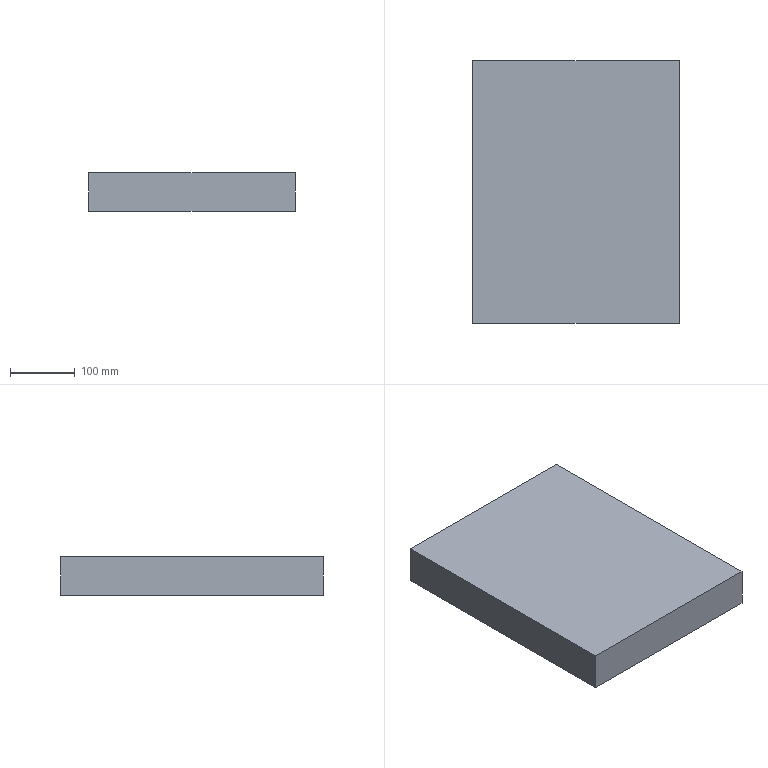Part | STEP file | zhichentai2 | 1 solid | 6 faces | box 320 x 406 x 60 mm | volume 7795200 mm3 | plane 6
STEP:
#1=CARTESIAN_POINT('',(0.,0.,0.));
#2=DIRECTION('',(0.,0.,1.));
#3=DIRECTION('',(1.,0.,0.));
#4=AXIS2_PLACEMENT_3D('',#1,#2,#3);
#5=CARTESIAN_POINT('',(160.,-203.,-30.));
#6=VERTEX_POINT('',#5);
#7=CARTESIAN_POINT('',(160.,203.,-30.));
#8=VERTEX_POINT('',#7);
#9=CARTESIAN_POINT('',(160.,203.,-30.));
#10=DIRECTION('',(0.,1.,0.));
#11=VECTOR('',#10,1.);
#12=LINE('',#9,#11);
#13=CARTESIAN_POINT('',(160.,203.,30.));
#14=DIRECTION('',(-1.,0.,0.));
#15=DIRECTION('',(0.,-1.,0.));
#16=AXIS2_PLACEMENT_3D('',#13,#14,#15);
#17=PLANE('',#16);
#18=CARTESIAN_POINT('',(0.,-60.));
#19=DIRECTION('',(-1.,0.));
#20=VECTOR('',#19,1.);
#21=LINE('',#18,#20);
#22=(GEOMETRIC_REPRESENTATION_CONTEXT(2)PARAMETRIC_REPRESENTATION_CONTEXT()REPRESENTATION_CONTEXT('',''));
#23=DEFINITIONAL_REPRESENTATION('',(#21),#22);
#24=PCURVE('',#17,#23);
#25=CARTESIAN_POINT('',(0.,0.,-30.));
#26=DIRECTION('',(0.,0.,1.));
#27=DIRECTION('',(1.,0.,0.));
#28=AXIS2_PLACEMENT_3D('',#25,#26,#27);
#29=PLANE('',#28);
#30=CARTESIAN_POINT('',(160.,203.));
#31=DIRECTION('',(0.,1.));
#32=VECTOR('',#31,1.);
#33=LINE('',#30,#32);
#34=(GEOMETRIC_REPRESENTATION_CONTEXT(2)PARAMETRIC_REPRESENTATION_CONTEXT()REPRESENTATION_CONTEXT('',''));
#35=DEFINITIONAL_REPRESENTATION('',(#33),#34);
#36=PCURVE('',#29,#35);
#37=SURFACE_CURVE('',#12,(#24,#36),.PCURVE_S1.);
#38=EDGE_CURVE('',#6,#8,#37,.T.);
#39=ORIENTED_EDGE('',*,*,#38,.T.);
#40=CARTESIAN_POINT('',(160.,203.,30.));
#41=VERTEX_POINT('',#40);
#42=CARTESIAN_POINT('',(160.,203.,30.));
#43=DIRECTION('',(0.,0.,-1.));
#44=VECTOR('',#43,1.);
#45=LINE('',#42,#44);
#46=CARTESIAN_POINT('',(0.,0.));
#47=DIRECTION('',(0.,-1.));
#48=VECTOR('',#47,1.);
#49=LINE('',#46,#48);
#50=(GEOMETRIC_REPRESENTATION_CONTEXT(2)PARAMETRIC_REPRESENTATION_CONTEXT()REPRESENTATION_CONTEXT('',''));
#51=DEFINITIONAL_REPRESENTATION('',(#49),#50);
#52=PCURVE('',#17,#51);
#53=CARTESIAN_POINT('',(-160.,203.,30.));
#54=DIRECTION('',(0.,-1.,0.));
#55=DIRECTION('',(0.,0.,-1.));
#56=AXIS2_PLACEMENT_3D('',#53,#54,#55);
#57=PLANE('',#56);
#58=CARTESIAN_POINT('',(0.,320.));
#59=DIRECTION('',(1.,0.));
#60=VECTOR('',#59,1.);
#61=LINE('',#58,#60);
#62=(GEOMETRIC_REPRESENTATION_CONTEXT(2)PARAMETRIC_REPRESENTATION_CONTEXT()REPRESENTATION_CONTEXT('',''));
#63=DEFINITIONAL_REPRESENTATION('',(#61),#62);
#64=PCURVE('',#57,#63);
#65=SURFACE_CURVE('',#45,(#52,#64),.PCURVE_S1.);
#66=EDGE_CURVE('',#41,#8,#65,.T.);
#67=ORIENTED_EDGE('',*,*,#66,.F.);
#68=CARTESIAN_POINT('',(160.,-203.,30.));
#69=VERTEX_POINT('',#68);
#70=CARTESIAN_POINT('',(160.,203.,30.));
#71=DIRECTION('',(0.,1.,0.));
#72=VECTOR('',#71,1.);
#73=LINE('',#70,#72);
#74=CARTESIAN_POINT('',(0.,0.));
#75=DIRECTION('',(-1.,0.));
#76=VECTOR('',#75,1.);
#77=LINE('',#74,#76);
#78=(GEOMETRIC_REPRESENTATION_CONTEXT(2)PARAMETRIC_REPRESENTATION_CONTEXT()REPRESENTATION_CONTEXT('',''));
#79=DEFINITIONAL_REPRESENTATION('',(#77),#78);
#80=PCURVE('',#17,#79);
#81=CARTESIAN_POINT('',(0.,0.,30.));
#82=DIRECTION('',(0.,0.,1.));
#83=DIRECTION('',(1.,0.,0.));
#84=AXIS2_PLACEMENT_3D('',#81,#82,#83);
#85=PLANE('',#84);
#86=CARTESIAN_POINT('',(160.,203.));
#87=DIRECTION('',(0.,1.));
#88=VECTOR('',#87,1.);
#89=LINE('',#86,#88);
#90=(GEOMETRIC_REPRESENTATION_CONTEXT(2)PARAMETRIC_REPRESENTATION_CONTEXT()REPRESENTATION_CONTEXT('',''));
#91=DEFINITIONAL_REPRESENTATION('',(#89),#90);
#92=PCURVE('',#85,#91);
#93=SURFACE_CURVE('',#73,(#80,#92),.PCURVE_S1.);
#94=EDGE_CURVE('',#69,#41,#93,.T.);
#95=ORIENTED_EDGE('',*,*,#94,.F.);
#96=CARTESIAN_POINT('',(160.,-203.,30.));
#97=DIRECTION('',(0.,0.,-1.));
#98=VECTOR('',#97,1.);
#99=LINE('',#96,#98);
#100=CARTESIAN_POINT('',(406.,0.));
#101=DIRECTION('',(0.,-1.));
#102=VECTOR('',#101,1.);
#103=LINE('',#100,#102);
#104=(GEOMETRIC_REPRESENTATION_CONTEXT(2)PARAMETRIC_REPRESENTATION_CONTEXT()REPRESENTATION_CONTEXT('',''));
#105=DEFINITIONAL_REPRESENTATION('',(#103),#104);
#106=PCURVE('',#17,#105);
#107=CARTESIAN_POINT('',(-160.,-203.,30.));
#108=DIRECTION('',(0.,1.,0.));
#109=DIRECTION('',(0.,0.,1.));
#110=AXIS2_PLACEMENT_3D('',#107,#108,#109);
#111=PLANE('',#110);
#112=CARTESIAN_POINT('',(0.,320.));
#113=DIRECTION('',(-1.,0.));
#114=VECTOR('',#113,1.);
#115=LINE('',#112,#114);
#116=(GEOMETRIC_REPRESENTATION_CONTEXT(2)PARAMETRIC_REPRESENTATION_CONTEXT()REPRESENTATION_CONTEXT('',''));
#117=DEFINITIONAL_REPRESENTATION('',(#115),#116);
#118=PCURVE('',#111,#117);
#119=SURFACE_CURVE('',#99,(#106,#118),.PCURVE_S1.);
#120=EDGE_CURVE('',#69,#6,#119,.T.);
#121=ORIENTED_EDGE('',*,*,#120,.T.);
#122=EDGE_LOOP('',(#39,#67,#95,#121));
#123=FACE_BOUND('',#122,.T.);
#124=ADVANCED_FACE('',(#123),#17,.F.);
#125=CARTESIAN_POINT('',(-160.,203.,-30.));
#126=VERTEX_POINT('',#125);
#127=CARTESIAN_POINT('',(-160.,203.,-30.));
#128=DIRECTION('',(-1.,0.,0.));
#129=VECTOR('',#128,1.);
#130=LINE('',#127,#129);
#131=CARTESIAN_POINT('',(60.,0.));
#132=DIRECTION('',(0.,-1.));
#133=VECTOR('',#132,1.);
#134=LINE('',#131,#133);
#135=(GEOMETRIC_REPRESENTATION_CONTEXT(2)PARAMETRIC_REPRESENTATION_CONTEXT()REPRESENTATION_CONTEXT('',''));
#136=DEFINITIONAL_REPRESENTATION('',(#134),#135);
#137=PCURVE('',#57,#136);
#138=CARTESIAN_POINT('',(-160.,203.));
#139=DIRECTION('',(-1.,0.));
#140=VECTOR('',#139,1.);
#141=LINE('',#138,#140);
#142=(GEOMETRIC_REPRESENTATION_CONTEXT(2)PARAMETRIC_REPRESENTATION_CONTEXT()REPRESENTATION_CONTEXT('',''));
#143=DEFINITIONAL_REPRESENTATION('',(#141),#142);
#144=PCURVE('',#29,#143);
#145=SURFACE_CURVE('',#130,(#137,#144),.PCURVE_S1.);
#146=EDGE_CURVE('',#8,#126,#145,.T.);
#147=ORIENTED_EDGE('',*,*,#146,.T.);
#148=CARTESIAN_POINT('',(-160.,203.,30.));
#149=VERTEX_POINT('',#148);
#150=CARTESIAN_POINT('',(-160.,203.,30.));
#151=DIRECTION('',(0.,0.,-1.));
#152=VECTOR('',#151,1.);
#153=LINE('',#150,#152);
#154=CARTESIAN_POINT('',(0.,0.));
#155=DIRECTION('',(1.,0.));
#156=VECTOR('',#155,1.);
#157=LINE('',#154,#156);
#158=(GEOMETRIC_REPRESENTATION_CONTEXT(2)PARAMETRIC_REPRESENTATION_CONTEXT()REPRESENTATION_CONTEXT('',''));
#159=DEFINITIONAL_REPRESENTATION('',(#157),#158);
#160=PCURVE('',#57,#159);
#161=CARTESIAN_POINT('',(-160.,203.,30.));
#162=DIRECTION('',(1.,0.,0.));
#163=DIRECTION('',(0.,1.,0.));
#164=AXIS2_PLACEMENT_3D('',#161,#162,#163);
#165=PLANE('',#164);
#166=CARTESIAN_POINT('',(0.,0.));
#167=DIRECTION('',(0.,-1.));
#168=VECTOR('',#167,1.);
#169=LINE('',#166,#168);
#170=(GEOMETRIC_REPRESENTATION_CONTEXT(2)PARAMETRIC_REPRESENTATION_CONTEXT()REPRESENTATION_CONTEXT('',''));
#171=DEFINITIONAL_REPRESENTATION('',(#169),#170);
#172=PCURVE('',#165,#171);
#173=SURFACE_CURVE('',#153,(#160,#172),.PCURVE_S1.);
#174=EDGE_CURVE('',#149,#126,#173,.T.);
#175=ORIENTED_EDGE('',*,*,#174,.F.);
#176=CARTESIAN_POINT('',(-160.,203.,30.));
#177=DIRECTION('',(-1.,0.,0.));
#178=VECTOR('',#177,1.);
#179=LINE('',#176,#178);
#180=CARTESIAN_POINT('',(0.,0.));
#181=DIRECTION('',(0.,-1.));
#182=VECTOR('',#181,1.);
#183=LINE('',#180,#182);
#184=(GEOMETRIC_REPRESENTATION_CONTEXT(2)PARAMETRIC_REPRESENTATION_CONTEXT()REPRESENTATION_CONTEXT('',''));
#185=DEFINITIONAL_REPRESENTATION('',(#183),#184);
#186=PCURVE('',#57,#185);
#187=CARTESIAN_POINT('',(-160.,203.));
#188=DIRECTION('',(-1.,0.));
#189=VECTOR('',#188,1.);
#190=LINE('',#187,#189);
#191=(GEOMETRIC_REPRESENTATION_CONTEXT(2)PARAMETRIC_REPRESENTATION_CONTEXT()REPRESENTATION_CONTEXT('',''));
#192=DEFINITIONAL_REPRESENTATION('',(#190),#191);
#193=PCURVE('',#85,#192);
#194=SURFACE_CURVE('',#179,(#186,#193),.PCURVE_S1.);
#195=EDGE_CURVE('',#41,#149,#194,.T.);
#196=ORIENTED_EDGE('',*,*,#195,.F.);
#197=ORIENTED_EDGE('',*,*,#66,.T.);
#198=EDGE_LOOP('',(#147,#175,#196,#197));
#199=FACE_BOUND('',#198,.T.);
#200=ADVANCED_FACE('',(#199),#57,.F.);
#201=CARTESIAN_POINT('',(-160.,-203.,-30.));
#202=VERTEX_POINT('',#201);
#203=CARTESIAN_POINT('',(-160.,203.,-30.));
#204=DIRECTION('',(0.,-1.,0.));
#205=VECTOR('',#204,1.);
#206=LINE('',#203,#205);
#207=CARTESIAN_POINT('',(0.,-60.));
#208=DIRECTION('',(-1.,0.));
#209=VECTOR('',#208,1.);
#210=LINE('',#207,#209);
#211=(GEOMETRIC_REPRESENTATION_CONTEXT(2)PARAMETRIC_REPRESENTATION_CONTEXT()REPRESENTATION_CONTEXT('',''));
#212=DEFINITIONAL_REPRESENTATION('',(#210),#211);
#213=PCURVE('',#165,#212);
#214=CARTESIAN_POINT('',(-160.,203.));
#215=DIRECTION('',(0.,-1.));
#216=VECTOR('',#215,1.);
#217=LINE('',#214,#216);
#218=(GEOMETRIC_REPRESENTATION_CONTEXT(2)PARAMETRIC_REPRESENTATION_CONTEXT()REPRESENTATION_CONTEXT('',''));
#219=DEFINITIONAL_REPRESENTATION('',(#217),#218);
#220=PCURVE('',#29,#219);
#221=SURFACE_CURVE('',#206,(#213,#220),.PCURVE_S1.);
#222=EDGE_CURVE('',#126,#202,#221,.T.);
#223=ORIENTED_EDGE('',*,*,#222,.T.);
#224=CARTESIAN_POINT('',(-160.,-203.,30.));
#225=VERTEX_POINT('',#224);
#226=CARTESIAN_POINT('',(-160.,-203.,30.));
#227=DIRECTION('',(0.,0.,-1.));
#228=VECTOR('',#227,1.);
#229=LINE('',#226,#228);
#230=CARTESIAN_POINT('',(-406.,0.));
#231=DIRECTION('',(0.,-1.));
#232=VECTOR('',#231,1.);
#233=LINE('',#230,#232);
#234=(GEOMETRIC_REPRESENTATION_CONTEXT(2)PARAMETRIC_REPRESENTATION_CONTEXT()REPRESENTATION_CONTEXT('',''));
#235=DEFINITIONAL_REPRESENTATION('',(#233),#234);
#236=PCURVE('',#165,#235);
#237=CARTESIAN_POINT('',(0.,0.));
#238=DIRECTION('',(-1.,0.));
#239=VECTOR('',#238,1.);
#240=LINE('',#237,#239);
#241=(GEOMETRIC_REPRESENTATION_CONTEXT(2)PARAMETRIC_REPRESENTATION_CONTEXT()REPRESENTATION_CONTEXT('',''));
#242=DEFINITIONAL_REPRESENTATION('',(#240),#241);
#243=PCURVE('',#111,#242);
#244=SURFACE_CURVE('',#229,(#236,#243),.PCURVE_S1.);
#245=EDGE_CURVE('',#225,#202,#244,.T.);
#246=ORIENTED_EDGE('',*,*,#245,.F.);
#247=CARTESIAN_POINT('',(-160.,203.,30.));
#248=DIRECTION('',(0.,-1.,0.));
#249=VECTOR('',#248,1.);
#250=LINE('',#247,#249);
#251=CARTESIAN_POINT('',(0.,0.));
#252=DIRECTION('',(-1.,0.));
#253=VECTOR('',#252,1.);
#254=LINE('',#251,#253);
#255=(GEOMETRIC_REPRESENTATION_CONTEXT(2)PARAMETRIC_REPRESENTATION_CONTEXT()REPRESENTATION_CONTEXT('',''));
#256=DEFINITIONAL_REPRESENTATION('',(#254),#255);
#257=PCURVE('',#165,#256);
#258=CARTESIAN_POINT('',(-160.,203.));
#259=DIRECTION('',(0.,-1.));
#260=VECTOR('',#259,1.);
#261=LINE('',#258,#260);
#262=(GEOMETRIC_REPRESENTATION_CONTEXT(2)PARAMETRIC_REPRESENTATION_CONTEXT()REPRESENTATION_CONTEXT('',''));
#263=DEFINITIONAL_REPRESENTATION('',(#261),#262);
#264=PCURVE('',#85,#263);
#265=SURFACE_CURVE('',#250,(#257,#264),.PCURVE_S1.);
#266=EDGE_CURVE('',#149,#225,#265,.T.);
#267=ORIENTED_EDGE('',*,*,#266,.F.);
#268=ORIENTED_EDGE('',*,*,#174,.T.);
#269=EDGE_LOOP('',(#223,#246,#267,#268));
#270=FACE_BOUND('',#269,.T.);
#271=ADVANCED_FACE('',(#270),#165,.F.);
#272=CARTESIAN_POINT('',(-160.,-203.,-30.));
#273=DIRECTION('',(1.,0.,0.));
#274=VECTOR('',#273,1.);
#275=LINE('',#272,#274);
#276=CARTESIAN_POINT('',(-60.,0.));
#277=DIRECTION('',(0.,1.));
#278=VECTOR('',#277,1.);
#279=LINE('',#276,#278);
#280=(GEOMETRIC_REPRESENTATION_CONTEXT(2)PARAMETRIC_REPRESENTATION_CONTEXT()REPRESENTATION_CONTEXT('',''));
#281=DEFINITIONAL_REPRESENTATION('',(#279),#280);
#282=PCURVE('',#111,#281);
#283=CARTESIAN_POINT('',(-160.,-203.));
#284=DIRECTION('',(1.,0.));
#285=VECTOR('',#284,1.);
#286=LINE('',#283,#285);
#287=(GEOMETRIC_REPRESENTATION_CONTEXT(2)PARAMETRIC_REPRESENTATION_CONTEXT()REPRESENTATION_CONTEXT('',''));
#288=DEFINITIONAL_REPRESENTATION('',(#286),#287);
#289=PCURVE('',#29,#288);
#290=SURFACE_CURVE('',#275,(#282,#289),.PCURVE_S1.);
#291=EDGE_CURVE('',#202,#6,#290,.T.);
#292=ORIENTED_EDGE('',*,*,#291,.T.);
#293=ORIENTED_EDGE('',*,*,#120,.F.);
#294=CARTESIAN_POINT('',(-160.,-203.,30.));
#295=DIRECTION('',(1.,0.,0.));
#296=VECTOR('',#295,1.);
#297=LINE('',#294,#296);
#298=CARTESIAN_POINT('',(0.,0.));
#299=DIRECTION('',(0.,1.));
#300=VECTOR('',#299,1.);
#301=LINE('',#298,#300);
#302=(GEOMETRIC_REPRESENTATION_CONTEXT(2)PARAMETRIC_REPRESENTATION_CONTEXT()REPRESENTATION_CONTEXT('',''));
#303=DEFINITIONAL_REPRESENTATION('',(#301),#302);
#304=PCURVE('',#111,#303);
#305=CARTESIAN_POINT('',(-160.,-203.));
#306=DIRECTION('',(1.,0.));
#307=VECTOR('',#306,1.);
#308=LINE('',#305,#307);
#309=(GEOMETRIC_REPRESENTATION_CONTEXT(2)PARAMETRIC_REPRESENTATION_CONTEXT()REPRESENTATION_CONTEXT('',''));
#310=DEFINITIONAL_REPRESENTATION('',(#308),#309);
#311=PCURVE('',#85,#310);
#312=SURFACE_CURVE('',#297,(#304,#311),.PCURVE_S1.);
#313=EDGE_CURVE('',#225,#69,#312,.T.);
#314=ORIENTED_EDGE('',*,*,#313,.F.);
#315=ORIENTED_EDGE('',*,*,#245,.T.);
#316=EDGE_LOOP('',(#292,#293,#314,#315));
#317=FACE_BOUND('',#316,.T.);
#318=ADVANCED_FACE('',(#317),#111,.F.);
#319=ORIENTED_EDGE('',*,*,#94,.T.);
#320=ORIENTED_EDGE('',*,*,#195,.T.);
#321=ORIENTED_EDGE('',*,*,#266,.T.);
#322=ORIENTED_EDGE('',*,*,#313,.T.);
#323=EDGE_LOOP('',(#319,#320,#321,#322));
#324=FACE_BOUND('',#323,.T.);
#325=ADVANCED_FACE('',(#324),#85,.T.);
#326=ORIENTED_EDGE('',*,*,#38,.F.);
#327=ORIENTED_EDGE('',*,*,#291,.F.);
#328=ORIENTED_EDGE('',*,*,#222,.F.);
#329=ORIENTED_EDGE('',*,*,#146,.F.);
#330=EDGE_LOOP('',(#326,#327,#328,#329));
#331=FACE_BOUND('',#330,.T.);
#332=ADVANCED_FACE('',(#331),#29,.F.);
#333=CLOSED_SHELL('',(#124,#200,#271,#318,#325,#332));
#334=MANIFOLD_SOLID_BREP('',#333);
#335=(LENGTH_UNIT()NAMED_UNIT(*)SI_UNIT(.MILLI.,.METRE.));
#336=UNCERTAINTY_MEASURE_WITH_UNIT(LENGTH_MEASURE(0.0000001),#335,'','');
#337=(NAMED_UNIT(*)PLANE_ANGLE_UNIT()SI_UNIT($,.RADIAN.));
#338=(NAMED_UNIT(*)SI_UNIT($,.STERADIAN.)SOLID_ANGLE_UNIT());
#339=(GEOMETRIC_REPRESENTATION_CONTEXT(3)GLOBAL_UNCERTAINTY_ASSIGNED_CONTEXT((#336))GLOBAL_UNIT_ASSIGNED_CONTEXT((#335,#337,#338))REPRESENTATION_CONTEXT('',''));
#340=ADVANCED_BREP_SHAPE_REPRESENTATION('',(#4,#334),#339);